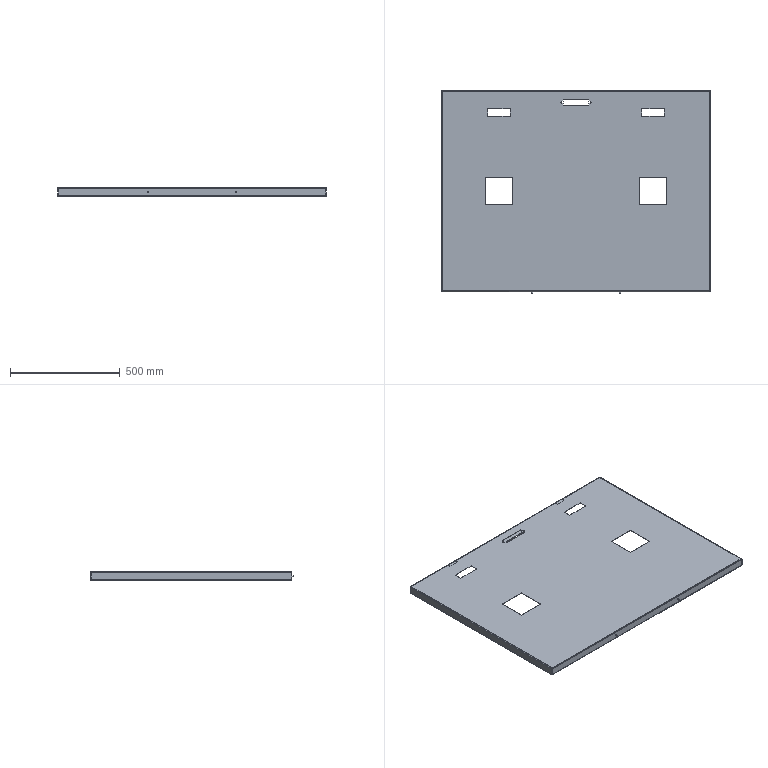Part | SolidWorks | features ICE 7, SMWeldBead 4, EdgeFlange 2, FlatPattern 1, HoleWzd 1, SMBaseFlange 1, SheetMetal 1 | 3 solids | 205 faces | box 1225 x 925 x 38 mm | volume 1989320 mm3 | plane 114 | cylinder 51 | spline 40 | commonest cylinder face diameters 3.3 x16 4 x12 7 x10 6 x6 2 x4 9 x3